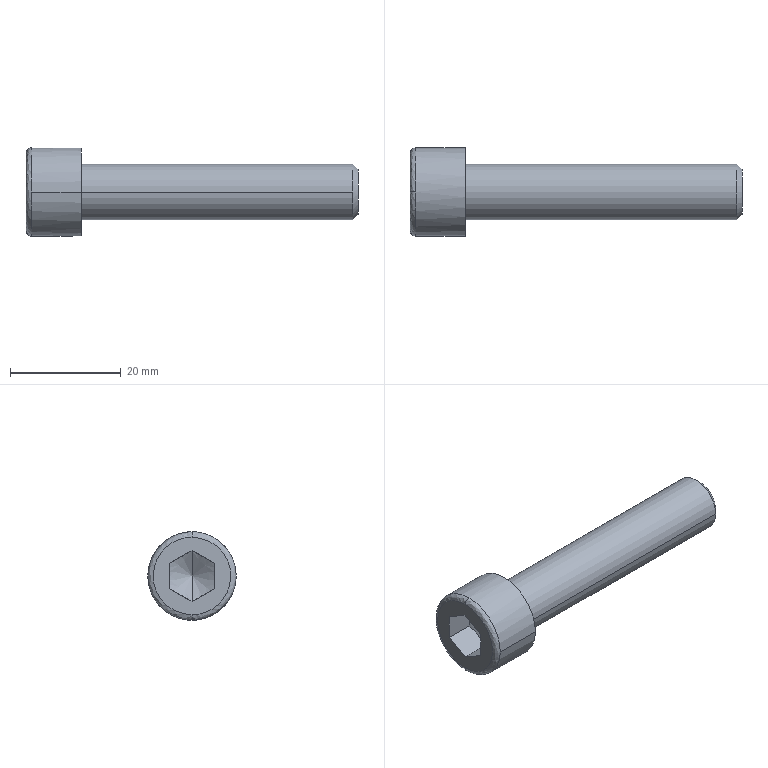Part | STEP file | DIN 912 - replaced by DIN EN ISO 4762 M10 x 50 | 1 solid | 21 faces | box 60 x 16 x 16 mm | volume 5580 mm3 | plane 9 | spline 4 | cylinder 4 | cone 4 | commonest cylinder face diameters 10 x2 16 x2